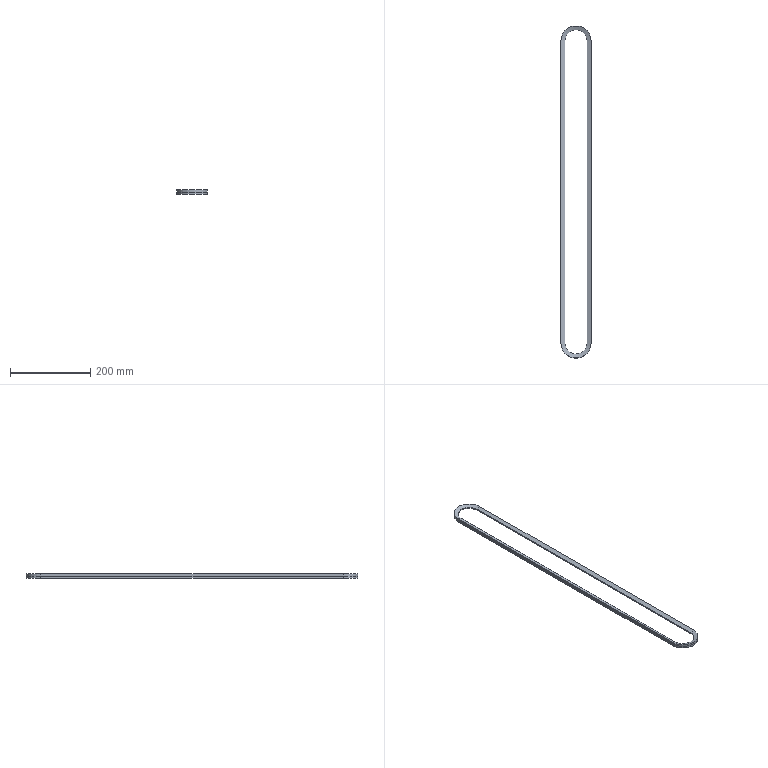Part | STEP file | 103000006127 | 1 solid | 24 faces | box 75 x 826 x 10 mm | volume 108901 mm3 | plane 12 | cylinder 8 | cone 4 | commonest cylinder face diameters 55 x4 75 x4
STEP:
#1=CARTESIAN_POINT('',(27.5,-751.,-1.36));
#2=VERTEX_POINT('',#1);
#3=CARTESIAN_POINT('',(37.5,-751.,-5.));
#4=VERTEX_POINT('',#3);
#5=CARTESIAN_POINT('',(32.5,-751.,-3.18));
#6=DIRECTION('',(0.9397,0.,-0.342));
#7=VECTOR('',#6,1.);
#8=LINE('',#5,#7);
#9=EDGE_CURVE('',#2,#4,#8,.T.);
#10=ORIENTED_EDGE('',*,*,#9,.F.);
#11=CARTESIAN_POINT('',(27.5,0.,-1.36));
#12=VERTEX_POINT('',#11);
#13=CARTESIAN_POINT('',(27.5,-375.5,-1.36));
#14=DIRECTION('',(0.,1.,0.));
#15=VECTOR('',#14,1.);
#16=LINE('',#13,#15);
#17=EDGE_CURVE('',#2,#12,#16,.T.);
#18=ORIENTED_EDGE('',*,*,#17,.T.);
#19=CARTESIAN_POINT('',(37.5,0.,-5.));
#20=VERTEX_POINT('',#19);
#21=CARTESIAN_POINT('',(32.5,0.,-3.18));
#22=DIRECTION('',(0.9397,0.,-0.342));
#23=VECTOR('',#22,1.);
#24=LINE('',#21,#23);
#25=EDGE_CURVE('',#12,#20,#24,.T.);
#26=ORIENTED_EDGE('',*,*,#25,.T.);
#27=CARTESIAN_POINT('',(37.5,-375.5,-5.));
#28=DIRECTION('',(0.,1.,0.));
#29=VECTOR('',#28,1.);
#30=LINE('',#27,#29);
#31=EDGE_CURVE('',#4,#20,#30,.T.);
#32=ORIENTED_EDGE('',*,*,#31,.F.);
#33=EDGE_LOOP('',(#10,#18,#26,#32));
#34=FACE_OUTER_BOUND('',#33,.T.);
#35=CARTESIAN_POINT('',(37.5,-751.,-5.));
#36=DIRECTION('',(0.342,0.,0.9397));
#37=DIRECTION('',(0.9397,0.,-0.342));
#38=AXIS2_PLACEMENT_3D('',#35,#36,#37);
#39=PLANE('',#38);
#40=ADVANCED_FACE('',(#34),#39,.F.);
#41=CARTESIAN_POINT('',(-37.5,-751.,-5.));
#42=VERTEX_POINT('',#41);
#43=CARTESIAN_POINT('',(0.,-751.,-5.));
#44=DIRECTION('',(0.,0.,-1.));
#45=AXIS2_PLACEMENT_3D('',#43,#44,$);
#46=CIRCLE('',#45,37.5);
#47=EDGE_CURVE('',#42,#4,#46,.F.);
#48=ORIENTED_EDGE('',*,*,#47,.F.);
#49=CARTESIAN_POINT('',(-27.5,-751.,-1.36));
#50=VERTEX_POINT('',#49);
#51=CARTESIAN_POINT('',(-469860.06,-751.,-171006.427));
#52=DIRECTION('',(-0.9397,0.,-0.342));
#53=VECTOR('',#52,1.);
#54=LINE('',#51,#53);
#55=EDGE_CURVE('',#50,#42,#54,.T.);
#56=ORIENTED_EDGE('',*,*,#55,.F.);
#57=CARTESIAN_POINT('',(0.,-751.,-1.36));
#58=DIRECTION('',(0.,0.,-1.));
#59=AXIS2_PLACEMENT_3D('',#57,#58,$);
#60=CIRCLE('',#59,27.5);
#61=EDGE_CURVE('',#50,#2,#60,.F.);
#62=ORIENTED_EDGE('',*,*,#61,.T.);
#63=ORIENTED_EDGE('',*,*,#9,.T.);
#64=EDGE_LOOP('',(#48,#56,#62,#63));
#65=FACE_OUTER_BOUND('',#64,.T.);
#66=CARTESIAN_POINT('',(0.,-751.,-1.36));
#67=DIRECTION('',(0.,0.,-1.));
#68=DIRECTION('',(1.,0.,0.));
#69=AXIS2_PLACEMENT_3D('',#66,#67,#68);
#70=CONICAL_SURFACE('',#69,27.5,1.222);
#71=ADVANCED_FACE('',(#65),#70,.F.);
#72=CARTESIAN_POINT('',(27.5,-751.,0.));
#73=VERTEX_POINT('',#72);
#74=CARTESIAN_POINT('',(27.5,0.,0.));
#75=VERTEX_POINT('',#74);
#76=CARTESIAN_POINT('',(27.5,-375.5,0.));
#77=DIRECTION('',(0.,1.,0.));
#78=VECTOR('',#77,1.);
#79=LINE('',#76,#78);
#80=EDGE_CURVE('',#73,#75,#79,.T.);
#81=ORIENTED_EDGE('',*,*,#80,.T.);
#82=CARTESIAN_POINT('',(27.5,0.,-0.6801));
#83=DIRECTION('',(0.,0.,-1.));
#84=VECTOR('',#83,1.);
#85=LINE('',#82,#84);
#86=EDGE_CURVE('',#75,#12,#85,.T.);
#87=ORIENTED_EDGE('',*,*,#86,.T.);
#88=ORIENTED_EDGE('',*,*,#17,.F.);
#89=CARTESIAN_POINT('',(27.5,-751.,-0.6801));
#90=DIRECTION('',(0.,0.,-1.));
#91=VECTOR('',#90,1.);
#92=LINE('',#89,#91);
#93=EDGE_CURVE('',#73,#2,#92,.T.);
#94=ORIENTED_EDGE('',*,*,#93,.F.);
#95=EDGE_LOOP('',(#81,#87,#88,#94));
#96=FACE_OUTER_BOUND('',#95,.T.);
#97=CARTESIAN_POINT('',(27.5,-751.,0.));
#98=DIRECTION('',(1.,0.,0.));
#99=DIRECTION('',(0.,1.,0.));
#100=AXIS2_PLACEMENT_3D('',#97,#98,#99);
#101=PLANE('',#100);
#102=ADVANCED_FACE('',(#96),#101,.F.);
#103=CARTESIAN_POINT('',(-37.5,0.,-5.));
#104=VERTEX_POINT('',#103);
#105=CARTESIAN_POINT('',(0.,0.,-5.));
#106=DIRECTION('',(0.,0.,-1.));
#107=AXIS2_PLACEMENT_3D('',#105,#106,$);
#108=CIRCLE('',#107,37.5);
#109=EDGE_CURVE('',#20,#104,#108,.F.);
#110=ORIENTED_EDGE('',*,*,#109,.F.);
#111=ORIENTED_EDGE('',*,*,#25,.F.);
#112=CARTESIAN_POINT('',(-27.5,0.,-1.36));
#113=VERTEX_POINT('',#112);
#114=CARTESIAN_POINT('',(0.,0.,-1.36));
#115=DIRECTION('',(0.,0.,-1.));
#116=AXIS2_PLACEMENT_3D('',#114,#115,$);
#117=CIRCLE('',#116,27.5);
#118=EDGE_CURVE('',#12,#113,#117,.F.);
#119=ORIENTED_EDGE('',*,*,#118,.T.);
#120=CARTESIAN_POINT('',(-469860.06,0.,-171006.427));
#121=DIRECTION('',(-0.9397,0.,-0.342));
#122=VECTOR('',#121,1.);
#123=LINE('',#120,#122);
#124=EDGE_CURVE('',#113,#104,#123,.T.);
#125=ORIENTED_EDGE('',*,*,#124,.T.);
#126=EDGE_LOOP('',(#110,#111,#119,#125));
#127=FACE_OUTER_BOUND('',#126,.T.);
#128=CARTESIAN_POINT('',(0.,0.,-1.36));
#129=DIRECTION('',(0.,0.,-1.));
#130=DIRECTION('',(-1.,0.,0.));
#131=AXIS2_PLACEMENT_3D('',#128,#129,#130);
#132=CONICAL_SURFACE('',#131,27.5,1.222);
#133=ADVANCED_FACE('',(#127),#132,.F.);
#134=ORIENTED_EDGE('',*,*,#31,.T.);
#135=CARTESIAN_POINT('',(37.5,0.,0.));
#136=VERTEX_POINT('',#135);
#137=CARTESIAN_POINT('',(37.5,0.,-2.5));
#138=DIRECTION('',(0.,0.,1.));
#139=VECTOR('',#138,1.);
#140=LINE('',#137,#139);
#141=EDGE_CURVE('',#20,#136,#140,.T.);
#142=ORIENTED_EDGE('',*,*,#141,.T.);
#143=CARTESIAN_POINT('',(37.5,-751.,0.));
#144=VERTEX_POINT('',#143);
#145=CARTESIAN_POINT('',(37.5,-375.5,0.));
#146=DIRECTION('',(0.,1.,0.));
#147=VECTOR('',#146,1.);
#148=LINE('',#145,#147);
#149=EDGE_CURVE('',#144,#136,#148,.T.);
#150=ORIENTED_EDGE('',*,*,#149,.F.);
#151=CARTESIAN_POINT('',(37.5,-751.,-2.5));
#152=DIRECTION('',(0.,0.,1.));
#153=VECTOR('',#152,1.);
#154=LINE('',#151,#153);
#155=EDGE_CURVE('',#4,#144,#154,.T.);
#156=ORIENTED_EDGE('',*,*,#155,.F.);
#157=EDGE_LOOP('',(#134,#142,#150,#156));
#158=FACE_OUTER_BOUND('',#157,.T.);
#159=CARTESIAN_POINT('',(37.5,-751.,0.));
#160=DIRECTION('',(-1.,0.,0.));
#161=DIRECTION('',(0.,-1.,0.));
#162=AXIS2_PLACEMENT_3D('',#159,#160,#161);
#163=PLANE('',#162);
#164=ADVANCED_FACE('',(#158),#163,.F.);
#165=CARTESIAN_POINT('',(-37.5,-751.,0.));
#166=VERTEX_POINT('',#165);
#167=CARTESIAN_POINT('',(0.,-751.,0.));
#168=DIRECTION('',(0.,0.,1.));
#169=AXIS2_PLACEMENT_3D('',#167,#168,$);
#170=CIRCLE('',#169,37.5);
#171=EDGE_CURVE('',#166,#144,#170,.T.);
#172=ORIENTED_EDGE('',*,*,#171,.F.);
#173=CARTESIAN_POINT('',(-37.5,-751.,0.));
#174=DIRECTION('',(0.,0.,1.));
#175=VECTOR('',#174,1.);
#176=LINE('',#173,#175);
#177=EDGE_CURVE('',#42,#166,#176,.T.);
#178=ORIENTED_EDGE('',*,*,#177,.F.);
#179=ORIENTED_EDGE('',*,*,#47,.T.);
#180=ORIENTED_EDGE('',*,*,#155,.T.);
#181=EDGE_LOOP('',(#172,#178,#179,#180));
#182=FACE_OUTER_BOUND('',#181,.T.);
#183=CARTESIAN_POINT('',(0.,-751.,0.));
#184=DIRECTION('',(0.,0.,1.));
#185=DIRECTION('',(-1.,0.,0.));
#186=AXIS2_PLACEMENT_3D('',#183,#184,#185);
#187=CYLINDRICAL_SURFACE('',#186,37.5);
#188=ADVANCED_FACE('',(#182),#187,.T.);
#189=CARTESIAN_POINT('',(-37.5,-375.5,-5.));
#190=DIRECTION('',(0.,-1.,0.));
#191=VECTOR('',#190,1.);
#192=LINE('',#189,#191);
#193=EDGE_CURVE('',#104,#42,#192,.T.);
#194=ORIENTED_EDGE('',*,*,#193,.F.);
#195=ORIENTED_EDGE('',*,*,#124,.F.);
#196=CARTESIAN_POINT('',(-27.5,-375.5,-1.36));
#197=DIRECTION('',(0.,-1.,0.));
#198=VECTOR('',#197,1.);
#199=LINE('',#196,#198);
#200=EDGE_CURVE('',#113,#50,#199,.T.);
#201=ORIENTED_EDGE('',*,*,#200,.T.);
#202=ORIENTED_EDGE('',*,*,#55,.T.);
#203=EDGE_LOOP('',(#194,#195,#201,#202));
#204=FACE_OUTER_BOUND('',#203,.T.);
#205=CARTESIAN_POINT('',(-37.5,0.,-5.));
#206=DIRECTION('',(-0.342,0.,0.9397));
#207=DIRECTION('',(0.9397,0.,0.342));
#208=AXIS2_PLACEMENT_3D('',#205,#206,#207);
#209=PLANE('',#208);
#210=ADVANCED_FACE('',(#204),#209,.F.);
#211=ORIENTED_EDGE('',*,*,#93,.T.);
#212=ORIENTED_EDGE('',*,*,#61,.F.);
#213=CARTESIAN_POINT('',(-27.5,-751.,0.));
#214=VERTEX_POINT('',#213);
#215=CARTESIAN_POINT('',(-27.5,-751.,0.));
#216=DIRECTION('',(0.,0.,1.));
#217=VECTOR('',#216,1.);
#218=LINE('',#215,#217);
#219=EDGE_CURVE('',#214,#50,#218,.F.);
#220=ORIENTED_EDGE('',*,*,#219,.F.);
#221=CARTESIAN_POINT('',(0.,-751.,0.));
#222=DIRECTION('',(0.,0.,1.));
#223=AXIS2_PLACEMENT_3D('',#221,#222,$);
#224=CIRCLE('',#223,27.5);
#225=EDGE_CURVE('',#214,#73,#224,.T.);
#226=ORIENTED_EDGE('',*,*,#225,.T.);
#227=EDGE_LOOP('',(#211,#212,#220,#226));
#228=FACE_OUTER_BOUND('',#227,.T.);
#229=CARTESIAN_POINT('',(0.,-751.,0.));
#230=DIRECTION('',(0.,0.,1.));
#231=DIRECTION('',(-1.,0.,0.));
#232=AXIS2_PLACEMENT_3D('',#229,#230,#231);
#233=CYLINDRICAL_SURFACE('',#232,27.5);
#234=ADVANCED_FACE('',(#228),#233,.F.);
#235=CARTESIAN_POINT('',(27.5,-751.,1.36));
#236=VERTEX_POINT('',#235);
#237=CARTESIAN_POINT('',(27.5,0.,1.36));
#238=VERTEX_POINT('',#237);
#239=CARTESIAN_POINT('',(27.5,-375.5,1.36));
#240=DIRECTION('',(0.,1.,0.));
#241=VECTOR('',#240,1.);
#242=LINE('',#239,#241);
#243=EDGE_CURVE('',#236,#238,#242,.T.);
#244=ORIENTED_EDGE('',*,*,#243,.T.);
#245=CARTESIAN_POINT('',(27.5,0.,0.6801));
#246=DIRECTION('',(0.,0.,-1.));
#247=VECTOR('',#246,1.);
#248=LINE('',#245,#247);
#249=EDGE_CURVE('',#238,#75,#248,.T.);
#250=ORIENTED_EDGE('',*,*,#249,.T.);
#251=ORIENTED_EDGE('',*,*,#80,.F.);
#252=CARTESIAN_POINT('',(27.5,-751.,0.6801));
#253=DIRECTION('',(0.,0.,-1.));
#254=VECTOR('',#253,1.);
#255=LINE('',#252,#254);
#256=EDGE_CURVE('',#236,#73,#255,.T.);
#257=ORIENTED_EDGE('',*,*,#256,.F.);
#258=EDGE_LOOP('',(#244,#250,#251,#257));
#259=FACE_OUTER_BOUND('',#258,.T.);
#260=CARTESIAN_POINT('',(27.5,-751.,0.));
#261=DIRECTION('',(1.,0.,0.));
#262=DIRECTION('',(0.,1.,0.));
#263=AXIS2_PLACEMENT_3D('',#260,#261,#262);
#264=PLANE('',#263);
#265=ADVANCED_FACE('',(#259),#264,.F.);
#266=CARTESIAN_POINT('',(-27.5,0.,0.));
#267=VERTEX_POINT('',#266);
#268=CARTESIAN_POINT('',(-27.5,0.,0.));
#269=DIRECTION('',(0.,0.,1.));
#270=VECTOR('',#269,1.);
#271=LINE('',#268,#270);
#272=EDGE_CURVE('',#267,#113,#271,.F.);
#273=ORIENTED_EDGE('',*,*,#272,.T.);
#274=ORIENTED_EDGE('',*,*,#118,.F.);
#275=ORIENTED_EDGE('',*,*,#86,.F.);
#276=CARTESIAN_POINT('',(0.,0.,0.));
#277=DIRECTION('',(0.,0.,1.));
#278=AXIS2_PLACEMENT_3D('',#276,#277,$);
#279=CIRCLE('',#278,27.5);
#280=EDGE_CURVE('',#75,#267,#279,.T.);
#281=ORIENTED_EDGE('',*,*,#280,.T.);
#282=EDGE_LOOP('',(#273,#274,#275,#281));
#283=FACE_OUTER_BOUND('',#282,.T.);
#284=CARTESIAN_POINT('',(0.,0.,0.));
#285=DIRECTION('',(0.,0.,1.));
#286=DIRECTION('',(1.,0.,0.));
#287=AXIS2_PLACEMENT_3D('',#284,#285,#286);
#288=CYLINDRICAL_SURFACE('',#287,27.5);
#289=ADVANCED_FACE('',(#283),#288,.F.);
#290=CARTESIAN_POINT('',(-37.5,0.,0.));
#291=VERTEX_POINT('',#290);
#292=CARTESIAN_POINT('',(0.,0.,0.));
#293=DIRECTION('',(0.,0.,1.));
#294=AXIS2_PLACEMENT_3D('',#292,#293,$);
#295=CIRCLE('',#294,37.5);
#296=EDGE_CURVE('',#136,#291,#295,.T.);
#297=ORIENTED_EDGE('',*,*,#296,.F.);
#298=ORIENTED_EDGE('',*,*,#141,.F.);
#299=ORIENTED_EDGE('',*,*,#109,.T.);
#300=CARTESIAN_POINT('',(-37.5,0.,0.));
#301=DIRECTION('',(0.,0.,1.));
#302=VECTOR('',#301,1.);
#303=LINE('',#300,#302);
#304=EDGE_CURVE('',#104,#291,#303,.T.);
#305=ORIENTED_EDGE('',*,*,#304,.T.);
#306=EDGE_LOOP('',(#297,#298,#299,#305));
#307=FACE_OUTER_BOUND('',#306,.T.);
#308=CARTESIAN_POINT('',(0.,0.,0.));
#309=DIRECTION('',(0.,0.,1.));
#310=DIRECTION('',(1.,0.,0.));
#311=AXIS2_PLACEMENT_3D('',#308,#309,#310);
#312=CYLINDRICAL_SURFACE('',#311,37.5);
#313=ADVANCED_FACE('',(#307),#312,.T.);
#314=ORIENTED_EDGE('',*,*,#149,.T.);
#315=CARTESIAN_POINT('',(37.5,0.,5.));
#316=VERTEX_POINT('',#315);
#317=CARTESIAN_POINT('',(37.5,0.,2.5));
#318=DIRECTION('',(0.,0.,1.));
#319=VECTOR('',#318,1.);
#320=LINE('',#317,#319);
#321=EDGE_CURVE('',#136,#316,#320,.T.);
#322=ORIENTED_EDGE('',*,*,#321,.T.);
#323=CARTESIAN_POINT('',(37.5,-751.,5.));
#324=VERTEX_POINT('',#323);
#325=CARTESIAN_POINT('',(37.5,-375.5,5.));
#326=DIRECTION('',(0.,1.,0.));
#327=VECTOR('',#326,1.);
#328=LINE('',#325,#327);
#329=EDGE_CURVE('',#324,#316,#328,.T.);
#330=ORIENTED_EDGE('',*,*,#329,.F.);
#331=CARTESIAN_POINT('',(37.5,-751.,2.5));
#332=DIRECTION('',(0.,0.,1.));
#333=VECTOR('',#332,1.);
#334=LINE('',#331,#333);
#335=EDGE_CURVE('',#144,#324,#334,.T.);
#336=ORIENTED_EDGE('',*,*,#335,.F.);
#337=EDGE_LOOP('',(#314,#322,#330,#336));
#338=FACE_OUTER_BOUND('',#337,.T.);
#339=CARTESIAN_POINT('',(37.5,-751.,0.));
#340=DIRECTION('',(-1.,0.,0.));
#341=DIRECTION('',(0.,-1.,0.));
#342=AXIS2_PLACEMENT_3D('',#339,#340,#341);
#343=PLANE('',#342);
#344=ADVANCED_FACE('',(#338),#343,.F.);
#345=CARTESIAN_POINT('',(-37.5,-751.,5.));
#346=VERTEX_POINT('',#345);
#347=CARTESIAN_POINT('',(0.,-751.,5.));
#348=DIRECTION('',(0.,0.,1.));
#349=AXIS2_PLACEMENT_3D('',#347,#348,$);
#350=CIRCLE('',#349,37.5);
#351=EDGE_CURVE('',#346,#324,#350,.T.);
#352=ORIENTED_EDGE('',*,*,#351,.F.);
#353=CARTESIAN_POINT('',(-37.5,-751.,0.));
#354=DIRECTION('',(0.,0.,1.));
#355=VECTOR('',#354,1.);
#356=LINE('',#353,#355);
#357=EDGE_CURVE('',#166,#346,#356,.T.);
#358=ORIENTED_EDGE('',*,*,#357,.F.);
#359=ORIENTED_EDGE('',*,*,#171,.T.);
#360=ORIENTED_EDGE('',*,*,#335,.T.);
#361=EDGE_LOOP('',(#352,#358,#359,#360));
#362=FACE_OUTER_BOUND('',#361,.T.);
#363=CARTESIAN_POINT('',(0.,-751.,0.));
#364=DIRECTION('',(0.,0.,1.));
#365=DIRECTION('',(-1.,0.,0.));
#366=AXIS2_PLACEMENT_3D('',#363,#364,#365);
#367=CYLINDRICAL_SURFACE('',#366,37.5);
#368=ADVANCED_FACE('',(#362),#367,.T.);
#369=CARTESIAN_POINT('',(-37.5,-375.5,0.));
#370=DIRECTION('',(0.,-1.,0.));
#371=VECTOR('',#370,1.);
#372=LINE('',#369,#371);
#373=EDGE_CURVE('',#291,#166,#372,.T.);
#374=ORIENTED_EDGE('',*,*,#373,.F.);
#375=ORIENTED_EDGE('',*,*,#304,.F.);
#376=ORIENTED_EDGE('',*,*,#193,.T.);
#377=ORIENTED_EDGE('',*,*,#177,.T.);
#378=EDGE_LOOP('',(#374,#375,#376,#377));
#379=FACE_OUTER_BOUND('',#378,.T.);
#380=CARTESIAN_POINT('',(-37.5,0.,0.));
#381=DIRECTION('',(1.,0.,0.));
#382=DIRECTION('',(0.,1.,0.));
#383=AXIS2_PLACEMENT_3D('',#380,#381,#382);
#384=PLANE('',#383);
#385=ADVANCED_FACE('',(#379),#384,.F.);
#386=ORIENTED_EDGE('',*,*,#219,.T.);
#387=ORIENTED_EDGE('',*,*,#200,.F.);
#388=ORIENTED_EDGE('',*,*,#272,.F.);
#389=CARTESIAN_POINT('',(-27.5,-375.5,0.));
#390=DIRECTION('',(0.,-1.,0.));
#391=VECTOR('',#390,1.);
#392=LINE('',#389,#391);
#393=EDGE_CURVE('',#267,#214,#392,.T.);
#394=ORIENTED_EDGE('',*,*,#393,.T.);
#395=EDGE_LOOP('',(#386,#387,#388,#394));
#396=FACE_OUTER_BOUND('',#395,.T.);
#397=CARTESIAN_POINT('',(-27.5,0.,0.));
#398=DIRECTION('',(-1.,0.,0.));
#399=DIRECTION('',(0.,-1.,0.));
#400=AXIS2_PLACEMENT_3D('',#397,#398,#399);
#401=PLANE('',#400);
#402=ADVANCED_FACE('',(#396),#401,.F.);
#403=ORIENTED_EDGE('',*,*,#225,.F.);
#404=CARTESIAN_POINT('',(-27.5,-751.,1.36));
#405=VERTEX_POINT('',#404);
#406=CARTESIAN_POINT('',(-27.5,-751.,0.));
#407=DIRECTION('',(0.,0.,1.));
#408=VECTOR('',#407,1.);
#409=LINE('',#406,#408);
#410=EDGE_CURVE('',#405,#214,#409,.F.);
#411=ORIENTED_EDGE('',*,*,#410,.F.);
#412=CARTESIAN_POINT('',(-27.5,-751.,1.36));
#413=CARTESIAN_POINT('',(-27.5,-755.32,1.36));
#414=CARTESIAN_POINT('',(-26.652,-759.639,1.36));
#415=CARTESIAN_POINT('',(-24.955,-763.737,1.36));
#416=CARTESIAN_POINT('',(-20.045,-771.045,1.36));
#417=CARTESIAN_POINT('',(-12.737,-775.955,1.36));
#418=CARTESIAN_POINT('',(-8.639,-777.652,1.36));
#419=CARTESIAN_POINT('',(0.,-779.348,1.36));
#420=CARTESIAN_POINT('',(8.639,-777.652,1.36));
#421=CARTESIAN_POINT('',(12.737,-775.955,1.36));
#422=CARTESIAN_POINT('',(20.045,-771.045,1.36));
#423=CARTESIAN_POINT('',(24.955,-763.737,1.36));
#424=CARTESIAN_POINT('',(26.652,-759.639,1.36));
#425=CARTESIAN_POINT('',(27.5,-755.32,1.36));
#426=CARTESIAN_POINT('',(27.5,-751.,1.36));
#427=B_SPLINE_CURVE_WITH_KNOTS('',5,(#412,#413,#414,#415,#416,#417,#418,#419,#420,#421,#422,#423,#424,#425,#426),.UNSPECIFIED.,.F.,.U.,(6,3,3,3,6),(-43.197,-21.598,0.,21.598,43.197),.UNSPECIFIED.);
#428=EDGE_CURVE('',#405,#236,#427,.T.);
#429=ORIENTED_EDGE('',*,*,#428,.T.);
#430=ORIENTED_EDGE('',*,*,#256,.T.);
#431=EDGE_LOOP('',(#403,#411,#429,#430));
#432=FACE_OUTER_BOUND('',#431,.T.);
#433=CARTESIAN_POINT('',(0.,-751.,0.));
#434=DIRECTION('',(0.,0.,1.));
#435=DIRECTION('',(-1.,0.,0.));
#436=AXIS2_PLACEMENT_3D('',#433,#434,#435);
#437=CYLINDRICAL_SURFACE('',#436,27.5);
#438=ADVANCED_FACE('',(#432),#437,.F.);
#439=ORIENTED_EDGE('',*,*,#329,.T.);
#440=CARTESIAN_POINT('',(32.5,0.,3.18));
#441=DIRECTION('',(-0.9397,0.,-0.342));
#442=VECTOR('',#441,1.);
#443=LINE('',#440,#442);
#444=EDGE_CURVE('',#316,#238,#443,.T.);
#445=ORIENTED_EDGE('',*,*,#444,.T.);
#446=ORIENTED_EDGE('',*,*,#243,.F.);
#447=CARTESIAN_POINT('',(32.5,-751.,3.18));
#448=DIRECTION('',(-0.9397,0.,-0.342));
#449=VECTOR('',#448,1.);
#450=LINE('',#447,#449);
#451=EDGE_CURVE('',#324,#236,#450,.T.);
#452=ORIENTED_EDGE('',*,*,#451,.F.);
#453=EDGE_LOOP('',(#439,#445,#446,#452));
#454=FACE_OUTER_BOUND('',#453,.T.);
#455=CARTESIAN_POINT('',(37.5,-751.,5.));
#456=DIRECTION('',(0.342,0.,-0.9397));
#457=DIRECTION('',(-0.9397,0.,-0.342));
#458=AXIS2_PLACEMENT_3D('',#455,#456,#457);
#459=PLANE('',#458);
#460=ADVANCED_FACE('',(#454),#459,.F.);
#461=ORIENTED_EDGE('',*,*,#280,.F.);
#462=ORIENTED_EDGE('',*,*,#249,.F.);
#463=CARTESIAN_POINT('',(-27.5,0.,1.36));
#464=VERTEX_POINT('',#463);
#465=CARTESIAN_POINT('',(0.,0.,1.36));
#466=DIRECTION('',(0.,0.,1.));
#467=AXIS2_PLACEMENT_3D('',#465,#466,$);
#468=CIRCLE('',#467,27.5);
#469=EDGE_CURVE('',#238,#464,#468,.T.);
#470=ORIENTED_EDGE('',*,*,#469,.T.);
#471=CARTESIAN_POINT('',(-27.5,0.,0.));
#472=DIRECTION('',(0.,0.,1.));
#473=VECTOR('',#472,1.);
#474=LINE('',#471,#473);
#475=EDGE_CURVE('',#464,#267,#474,.F.);
#476=ORIENTED_EDGE('',*,*,#475,.T.);
#477=EDGE_LOOP('',(#461,#462,#470,#476));
#478=FACE_OUTER_BOUND('',#477,.T.);
#479=CARTESIAN_POINT('',(0.,0.,0.));
#480=DIRECTION('',(0.,0.,1.));
#481=DIRECTION('',(1.,0.,0.));
#482=AXIS2_PLACEMENT_3D('',#479,#480,#481);
#483=CYLINDRICAL_SURFACE('',#482,27.5);
#484=ADVANCED_FACE('',(#478),#483,.F.);
#485=CARTESIAN_POINT('',(-37.5,0.,5.));
#486=VERTEX_POINT('',#485);
#487=CARTESIAN_POINT('',(0.,0.,5.));
#488=DIRECTION('',(0.,0.,1.));
#489=AXIS2_PLACEMENT_3D('',#487,#488,$);
#490=CIRCLE('',#489,37.5);
#491=EDGE_CURVE('',#316,#486,#490,.T.);
#492=ORIENTED_EDGE('',*,*,#491,.F.);
#493=ORIENTED_EDGE('',*,*,#321,.F.);
#494=ORIENTED_EDGE('',*,*,#296,.T.);
#495=CARTESIAN_POINT('',(-37.5,0.,0.));
#496=DIRECTION('',(0.,0.,1.));
#497=VECTOR('',#496,1.);
#498=LINE('',#495,#497);
#499=EDGE_CURVE('',#291,#486,#498,.T.);
#500=ORIENTED_EDGE('',*,*,#499,.T.);
#501=EDGE_LOOP('',(#492,#493,#494,#500));
#502=FACE_OUTER_BOUND('',#501,.T.);
#503=CARTESIAN_POINT('',(0.,0.,0.));
#504=DIRECTION('',(0.,0.,1.));
#505=DIRECTION('',(1.,0.,0.));
#506=AXIS2_PLACEMENT_3D('',#503,#504,#505);
#507=CYLINDRICAL_SURFACE('',#506,37.5);
#508=ADVANCED_FACE('',(#502),#507,.T.);
#509=ORIENTED_EDGE('',*,*,#428,.F.);
#510=CARTESIAN_POINT('',(-469865.06,-751.,171008.247));
#511=DIRECTION('',(-0.9397,0.,0.342));
#512=VECTOR('',#511,1.);
#513=LINE('',#510,#512);
#514=EDGE_CURVE('',#346,#405,#513,.F.);
#515=ORIENTED_EDGE('',*,*,#514,.F.);
#516=ORIENTED_EDGE('',*,*,#351,.T.);
#517=ORIENTED_EDGE('',*,*,#451,.T.);
#518=EDGE_LOOP('',(#509,#515,#516,#517));
#519=FACE_OUTER_BOUND('',#518,.T.);
#520=CARTESIAN_POINT('',(0.,-751.,5.));
#521=DIRECTION('',(0.,0.,1.));
#522=DIRECTION('',(-1.,0.,0.));
#523=AXIS2_PLACEMENT_3D('',#520,#521,#522);
#524=CONICAL_SURFACE('',#523,37.5,1.222);
#525=ADVANCED_FACE('',(#519),#524,.F.);
#526=CARTESIAN_POINT('',(-37.5,-375.5,5.));
#527=DIRECTION('',(0.,-1.,0.));
#528=VECTOR('',#527,1.);
#529=LINE('',#526,#528);
#530=EDGE_CURVE('',#486,#346,#529,.T.);
#531=ORIENTED_EDGE('',*,*,#530,.F.);
#532=ORIENTED_EDGE('',*,*,#499,.F.);
#533=ORIENTED_EDGE('',*,*,#373,.T.);
#534=ORIENTED_EDGE('',*,*,#357,.T.);
#535=EDGE_LOOP('',(#531,#532,#533,#534));
#536=FACE_OUTER_BOUND('',#535,.T.);
#537=CARTESIAN_POINT('',(-37.5,0.,0.));
#538=DIRECTION('',(1.,0.,0.));
#539=DIRECTION('',(0.,1.,0.));
#540=AXIS2_PLACEMENT_3D('',#537,#538,#539);
#541=PLANE('',#540);
#542=ADVANCED_FACE('',(#536),#541,.F.);
#543=ORIENTED_EDGE('',*,*,#393,.F.);
#544=ORIENTED_EDGE('',*,*,#475,.F.);
#545=CARTESIAN_POINT('',(-27.5,-375.5,1.36));
#546=DIRECTION('',(0.,-1.,0.));
#547=VECTOR('',#546,1.);
#548=LINE('',#545,#547);
#549=EDGE_CURVE('',#464,#405,#548,.T.);
#550=ORIENTED_EDGE('',*,*,#549,.T.);
#551=ORIENTED_EDGE('',*,*,#410,.T.);
#552=EDGE_LOOP('',(#543,#544,#550,#551));
#553=FACE_OUTER_BOUND('',#552,.T.);
#554=CARTESIAN_POINT('',(-27.5,0.,0.));
#555=DIRECTION('',(-1.,0.,0.));
#556=DIRECTION('',(0.,-1.,0.));
#557=AXIS2_PLACEMENT_3D('',#554,#555,#556);
#558=PLANE('',#557);
#559=ADVANCED_FACE('',(#553),#558,.F.);
#560=ORIENTED_EDGE('',*,*,#469,.F.);
#561=ORIENTED_EDGE('',*,*,#444,.F.);
#562=ORIENTED_EDGE('',*,*,#491,.T.);
#563=CARTESIAN_POINT('',(-469865.06,0.,171008.247));
#564=DIRECTION('',(-0.9397,0.,0.342));
#565=VECTOR('',#564,1.);
#566=LINE('',#563,#565);
#567=EDGE_CURVE('',#486,#464,#566,.F.);
#568=ORIENTED_EDGE('',*,*,#567,.T.);
#569=EDGE_LOOP('',(#560,#561,#562,#568));
#570=FACE_OUTER_BOUND('',#569,.T.);
#571=CARTESIAN_POINT('',(0.,0.,5.));
#572=DIRECTION('',(0.,0.,1.));
#573=DIRECTION('',(1.,0.,0.));
#574=AXIS2_PLACEMENT_3D('',#571,#572,#573);
#575=CONICAL_SURFACE('',#574,37.5,1.222);
#576=ADVANCED_FACE('',(#570),#575,.F.);
#577=ORIENTED_EDGE('',*,*,#549,.F.);
#578=ORIENTED_EDGE('',*,*,#567,.F.);
#579=ORIENTED_EDGE('',*,*,#530,.T.);
#580=ORIENTED_EDGE('',*,*,#514,.T.);
#581=EDGE_LOOP('',(#577,#578,#579,#580));
#582=FACE_OUTER_BOUND('',#581,.T.);
#583=CARTESIAN_POINT('',(-37.5,0.,5.));
#584=DIRECTION('',(-0.342,0.,-0.9397));
#585=DIRECTION('',(-0.9397,0.,0.342));
#586=AXIS2_PLACEMENT_3D('',#583,#584,#585);
#587=PLANE('',#586);
#588=ADVANCED_FACE('',(#582),#587,.F.);
#589=CLOSED_SHELL('',(#40,#71,#102,#133,#164,#188,#210,#234,#265,#289,#313,#344,#368,#385,#402,#438,#460,#484,#508,#525,#542,#559,#576,#588));
#590=MANIFOLD_SOLID_BREP('',#589);
#591=(LENGTH_UNIT()NAMED_UNIT(*)SI_UNIT(.MILLI.,.METRE.));
#592=UNCERTAINTY_MEASURE_WITH_UNIT(LENGTH_MEASURE(0.005),#591,'','');
#593=(NAMED_UNIT(*)PLANE_ANGLE_UNIT()SI_UNIT($,.RADIAN.));
#594=(NAMED_UNIT(*)SI_UNIT($,.STERADIAN.)SOLID_ANGLE_UNIT());
#595=(GEOMETRIC_REPRESENTATION_CONTEXT(3)GLOBAL_UNCERTAINTY_ASSIGNED_CONTEXT((#592))GLOBAL_UNIT_ASSIGNED_CONTEXT((#591,#593,#594))REPRESENTATION_CONTEXT('',''));
#596=ADVANCED_BREP_SHAPE_REPRESENTATION('',(#590),#595);